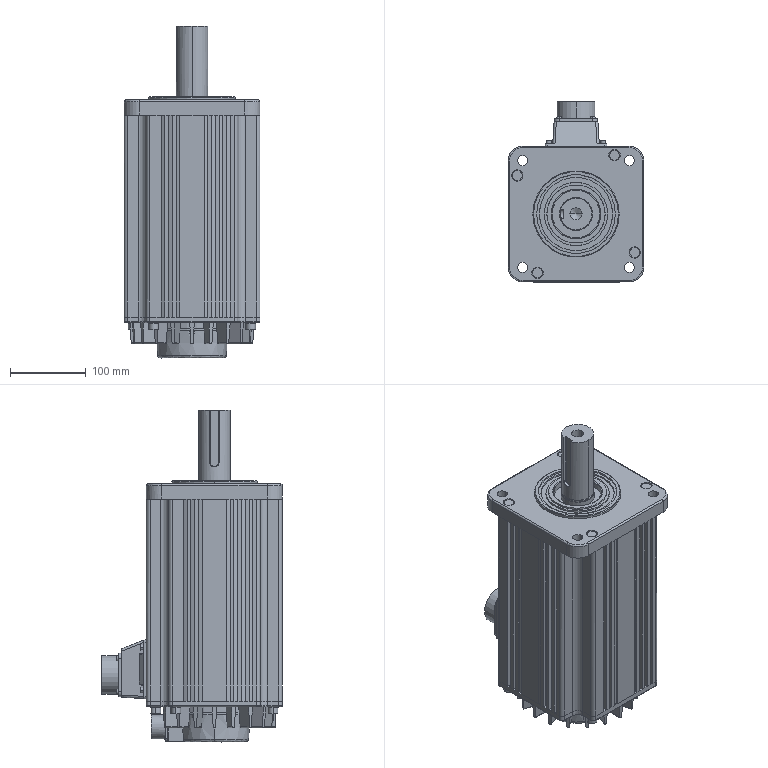Part | SolidWorks | features BaseBody 1 | 1 solid | 2176 faces | box 180 x 239.2 x 439.7 mm | volume 9178277 mm3 | plane 1387 | spline 543 | cylinder 203 | cone 39 | torus 4 | commonest cylinder face diameters 8 x24 180 x21 2 x20 3.23 x17 10 x16 13 x16